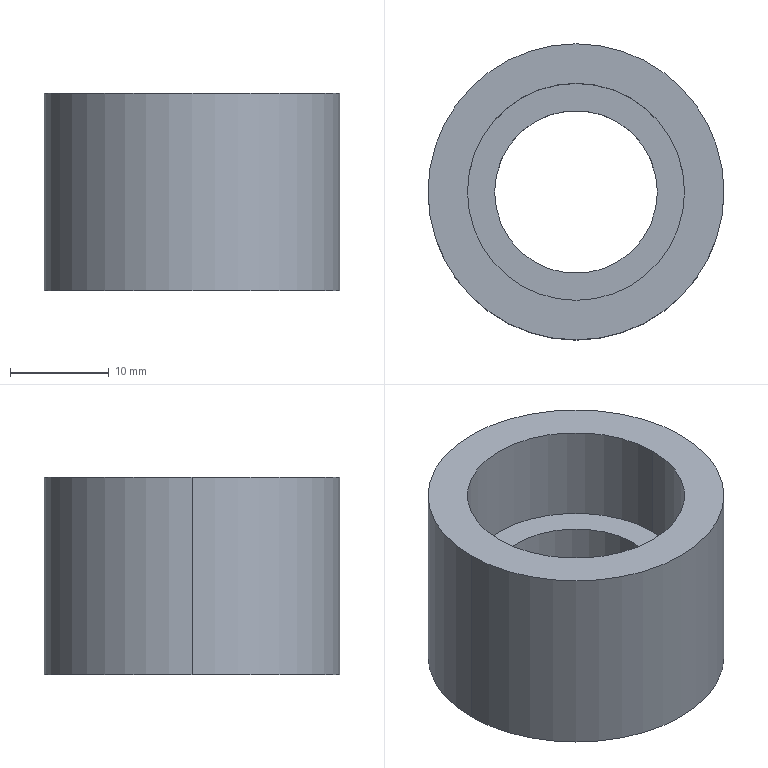Part | SolidWorks | features Extrusion 1, HoleWzd 1, ICE 1 | 1 solid | 9 faces | box 30 x 30 x 20 mm | volume 8198 mm3 | cylinder 6 | plane 3 | commonest cylinder face diameters 16.5 x2 22 x2 30 x2
STEP:
#1=CARTESIAN_POINT('',(-8.25,0.,10.));
#2=VERTEX_POINT('',#1);
#3=CARTESIAN_POINT('',(8.25,0.,10.));
#4=VERTEX_POINT('',#3);
#5=CARTESIAN_POINT('',(0.,0.,10.));
#6=DIRECTION('',(0.,0.,1.));
#7=DIRECTION('',(1.,0.,0.));
#8=AXIS2_PLACEMENT_3D('',#5,#6,#7);
#9=CIRCLE('',#8,8.25);
#10=EDGE_CURVE('',#2,#4,#9,.T.);
#11=ORIENTED_EDGE('',*,*,#10,.T.);
#12=CARTESIAN_POINT('',(8.25,0.,0.));
#13=VERTEX_POINT('',#12);
#14=CARTESIAN_POINT('',(8.25,0.,0.));
#15=DIRECTION('',(0.,0.,-1.));
#16=VECTOR('',#15,1000.);
#17=LINE('',#14,#16);
#18=EDGE_CURVE('',#4,#13,#17,.T.);
#19=ORIENTED_EDGE('',*,*,#18,.T.);
#20=CARTESIAN_POINT('',(-8.25,0.,0.));
#21=VERTEX_POINT('',#20);
#22=CARTESIAN_POINT('',(0.,0.,0.));
#23=DIRECTION('',(0.,0.,-1.));
#24=DIRECTION('',(-1.,0.,0.));
#25=AXIS2_PLACEMENT_3D('',#22,#23,#24);
#26=CIRCLE('',#25,8.25);
#27=EDGE_CURVE('',#13,#21,#26,.T.);
#28=ORIENTED_EDGE('',*,*,#27,.T.);
#29=CARTESIAN_POINT('',(-8.25,0.,0.));
#30=DIRECTION('',(0.,0.,-1.));
#31=VECTOR('',#30,1000.);
#32=LINE('',#29,#31);
#33=EDGE_CURVE('',#2,#21,#32,.T.);
#34=ORIENTED_EDGE('',*,*,#33,.F.);
#35=EDGE_LOOP('',(#11,#19,#28,#34));
#36=FACE_OUTER_BOUND('',#35,.T.);
#37=CARTESIAN_POINT('',(0.,0.,0.));
#38=DIRECTION('',(0.,0.,-1.));
#39=DIRECTION('',(-1.,0.,0.));
#40=AXIS2_PLACEMENT_3D('',#37,#38,#39);
#41=CYLINDRICAL_SURFACE('',#40,8.25);
#42=ADVANCED_FACE('',(#36),#41,.F.);
#43=CARTESIAN_POINT('',(-11.,0.,10.));
#44=VERTEX_POINT('',#43);
#45=CARTESIAN_POINT('',(11.,0.,10.));
#46=VERTEX_POINT('',#45);
#47=CARTESIAN_POINT('',(0.,0.,10.));
#48=DIRECTION('',(0.,0.,1.));
#49=DIRECTION('',(1.,0.,0.));
#50=AXIS2_PLACEMENT_3D('',#47,#48,#49);
#51=CIRCLE('',#50,11.);
#52=EDGE_CURVE('',#44,#46,#51,.T.);
#53=ORIENTED_EDGE('',*,*,#52,.F.);
#54=CARTESIAN_POINT('',(-11.,0.,20.));
#55=VERTEX_POINT('',#54);
#56=CARTESIAN_POINT('',(-11.,0.,10.));
#57=DIRECTION('',(0.,0.,1.));
#58=VECTOR('',#57,1000.);
#59=LINE('',#56,#58);
#60=EDGE_CURVE('',#44,#55,#59,.T.);
#61=ORIENTED_EDGE('',*,*,#60,.T.);
#62=CARTESIAN_POINT('',(11.,0.,20.));
#63=VERTEX_POINT('',#62);
#64=CARTESIAN_POINT('',(0.,0.,20.));
#65=DIRECTION('',(0.,0.,1.));
#66=DIRECTION('',(1.,0.,0.));
#67=AXIS2_PLACEMENT_3D('',#64,#65,#66);
#68=CIRCLE('',#67,11.);
#69=EDGE_CURVE('',#55,#63,#68,.T.);
#70=ORIENTED_EDGE('',*,*,#69,.T.);
#71=CARTESIAN_POINT('',(11.,0.,10.));
#72=DIRECTION('',(0.,0.,1.));
#73=VECTOR('',#72,1000.);
#74=LINE('',#71,#73);
#75=EDGE_CURVE('',#46,#63,#74,.T.);
#76=ORIENTED_EDGE('',*,*,#75,.F.);
#77=EDGE_LOOP('',(#53,#61,#70,#76));
#78=FACE_OUTER_BOUND('',#77,.T.);
#79=CARTESIAN_POINT('',(0.,0.,10.));
#80=DIRECTION('',(0.,0.,1.));
#81=DIRECTION('',(1.,0.,0.));
#82=AXIS2_PLACEMENT_3D('',#79,#80,#81);
#83=CYLINDRICAL_SURFACE('',#82,11.);
#84=ADVANCED_FACE('',(#78),#83,.F.);
#85=CARTESIAN_POINT('',(15.,0.,20.));
#86=VERTEX_POINT('',#85);
#87=CARTESIAN_POINT('',(-15.,0.,20.));
#88=VERTEX_POINT('',#87);
#89=CARTESIAN_POINT('',(0.,0.,20.));
#90=DIRECTION('',(0.,0.,1.));
#91=DIRECTION('',(1.,0.,0.));
#92=AXIS2_PLACEMENT_3D('',#89,#90,#91);
#93=CIRCLE('',#92,15.);
#94=EDGE_CURVE('',#86,#88,#93,.T.);
#95=ORIENTED_EDGE('',*,*,#94,.F.);
#96=CARTESIAN_POINT('',(15.,0.,0.));
#97=VERTEX_POINT('',#96);
#98=CARTESIAN_POINT('',(15.,0.,20.));
#99=DIRECTION('',(0.,0.,-1.));
#100=VECTOR('',#99,1000.);
#101=LINE('',#98,#100);
#102=EDGE_CURVE('',#86,#97,#101,.T.);
#103=ORIENTED_EDGE('',*,*,#102,.T.);
#104=CARTESIAN_POINT('',(-15.,0.,0.));
#105=VERTEX_POINT('',#104);
#106=CARTESIAN_POINT('',(0.,0.,0.));
#107=DIRECTION('',(0.,0.,1.));
#108=DIRECTION('',(1.,0.,0.));
#109=AXIS2_PLACEMENT_3D('',#106,#107,#108);
#110=CIRCLE('',#109,15.);
#111=EDGE_CURVE('',#97,#105,#110,.T.);
#112=ORIENTED_EDGE('',*,*,#111,.T.);
#113=CARTESIAN_POINT('',(-15.,0.,20.));
#114=DIRECTION('',(0.,0.,-1.));
#115=VECTOR('',#114,1000.);
#116=LINE('',#113,#115);
#117=EDGE_CURVE('',#88,#105,#116,.T.);
#118=ORIENTED_EDGE('',*,*,#117,.F.);
#119=EDGE_LOOP('',(#95,#103,#112,#118));
#120=FACE_OUTER_BOUND('',#119,.T.);
#121=CARTESIAN_POINT('',(0.,0.,20.));
#122=DIRECTION('',(0.,0.,-1.));
#123=DIRECTION('',(-1.,0.,0.));
#124=AXIS2_PLACEMENT_3D('',#121,#122,#123);
#125=CYLINDRICAL_SURFACE('',#124,15.);
#126=ADVANCED_FACE('',(#120),#125,.T.);
#127=ORIENTED_EDGE('',*,*,#102,.F.);
#128=CARTESIAN_POINT('',(0.,0.,20.));
#129=DIRECTION('',(0.,0.,1.));
#130=DIRECTION('',(1.,0.,0.));
#131=AXIS2_PLACEMENT_3D('',#128,#129,#130);
#132=CIRCLE('',#131,15.);
#133=EDGE_CURVE('',#88,#86,#132,.T.);
#134=ORIENTED_EDGE('',*,*,#133,.F.);
#135=ORIENTED_EDGE('',*,*,#117,.T.);
#136=CARTESIAN_POINT('',(0.,0.,0.));
#137=DIRECTION('',(0.,0.,1.));
#138=DIRECTION('',(1.,0.,0.));
#139=AXIS2_PLACEMENT_3D('',#136,#137,#138);
#140=CIRCLE('',#139,15.);
#141=EDGE_CURVE('',#105,#97,#140,.T.);
#142=ORIENTED_EDGE('',*,*,#141,.T.);
#143=EDGE_LOOP('',(#127,#134,#135,#142));
#144=FACE_OUTER_BOUND('',#143,.T.);
#145=CARTESIAN_POINT('',(0.,0.,20.));
#146=DIRECTION('',(0.,0.,-1.));
#147=DIRECTION('',(-1.,0.,0.));
#148=AXIS2_PLACEMENT_3D('',#145,#146,#147);
#149=CYLINDRICAL_SURFACE('',#148,15.);
#150=ADVANCED_FACE('',(#144),#149,.T.);
#151=CARTESIAN_POINT('',(0.,0.,20.));
#152=DIRECTION('',(0.,0.,1.));
#153=DIRECTION('',(1.,0.,0.));
#154=AXIS2_PLACEMENT_3D('',#151,#152,#153);
#155=CIRCLE('',#154,11.);
#156=EDGE_CURVE('',#63,#55,#155,.T.);
#157=ORIENTED_EDGE('',*,*,#156,.F.);
#158=ORIENTED_EDGE('',*,*,#69,.F.);
#159=EDGE_LOOP('',(#157,#158));
#160=FACE_BOUND('',#159,.T.);
#161=ORIENTED_EDGE('',*,*,#133,.T.);
#162=ORIENTED_EDGE('',*,*,#94,.T.);
#163=EDGE_LOOP('',(#161,#162));
#164=FACE_OUTER_BOUND('',#163,.T.);
#165=CARTESIAN_POINT('',(0.,0.,20.));
#166=DIRECTION('',(0.,0.,1.));
#167=DIRECTION('',(1.,0.,0.));
#168=AXIS2_PLACEMENT_3D('',#165,#166,#167);
#169=PLANE('',#168);
#170=ADVANCED_FACE('',(#160,#164),#169,.T.);
#171=CARTESIAN_POINT('',(0.,0.,0.));
#172=DIRECTION('',(0.,0.,-1.));
#173=DIRECTION('',(-1.,0.,0.));
#174=AXIS2_PLACEMENT_3D('',#171,#172,#173);
#175=CIRCLE('',#174,8.25);
#176=EDGE_CURVE('',#21,#13,#175,.T.);
#177=ORIENTED_EDGE('',*,*,#176,.F.);
#178=ORIENTED_EDGE('',*,*,#27,.F.);
#179=EDGE_LOOP('',(#177,#178));
#180=FACE_BOUND('',#179,.T.);
#181=ORIENTED_EDGE('',*,*,#141,.F.);
#182=ORIENTED_EDGE('',*,*,#111,.F.);
#183=EDGE_LOOP('',(#181,#182));
#184=FACE_OUTER_BOUND('',#183,.T.);
#185=CARTESIAN_POINT('',(0.,0.,0.));
#186=DIRECTION('',(0.,0.,1.));
#187=DIRECTION('',(1.,0.,0.));
#188=AXIS2_PLACEMENT_3D('',#185,#186,#187);
#189=PLANE('',#188);
#190=ADVANCED_FACE('',(#180,#184),#189,.F.);
#191=ORIENTED_EDGE('',*,*,#60,.F.);
#192=CARTESIAN_POINT('',(0.,0.,10.));
#193=DIRECTION('',(0.,0.,1.));
#194=DIRECTION('',(1.,0.,0.));
#195=AXIS2_PLACEMENT_3D('',#192,#193,#194);
#196=CIRCLE('',#195,11.);
#197=EDGE_CURVE('',#46,#44,#196,.T.);
#198=ORIENTED_EDGE('',*,*,#197,.F.);
#199=ORIENTED_EDGE('',*,*,#75,.T.);
#200=ORIENTED_EDGE('',*,*,#156,.T.);
#201=EDGE_LOOP('',(#191,#198,#199,#200));
#202=FACE_OUTER_BOUND('',#201,.T.);
#203=CARTESIAN_POINT('',(0.,0.,10.));
#204=DIRECTION('',(0.,0.,1.));
#205=DIRECTION('',(1.,0.,0.));
#206=AXIS2_PLACEMENT_3D('',#203,#204,#205);
#207=CYLINDRICAL_SURFACE('',#206,11.);
#208=ADVANCED_FACE('',(#202),#207,.F.);
#209=ORIENTED_EDGE('',*,*,#10,.F.);
#210=CARTESIAN_POINT('',(0.,0.,10.));
#211=DIRECTION('',(0.,0.,1.));
#212=DIRECTION('',(1.,0.,0.));
#213=AXIS2_PLACEMENT_3D('',#210,#211,#212);
#214=CIRCLE('',#213,8.25);
#215=EDGE_CURVE('',#4,#2,#214,.T.);
#216=ORIENTED_EDGE('',*,*,#215,.F.);
#217=EDGE_LOOP('',(#209,#216));
#218=FACE_BOUND('',#217,.T.);
#219=ORIENTED_EDGE('',*,*,#197,.T.);
#220=ORIENTED_EDGE('',*,*,#52,.T.);
#221=EDGE_LOOP('',(#219,#220));
#222=FACE_OUTER_BOUND('',#221,.T.);
#223=CARTESIAN_POINT('',(0.,0.,10.));
#224=DIRECTION('',(0.,0.,1.));
#225=DIRECTION('',(1.,0.,0.));
#226=AXIS2_PLACEMENT_3D('',#223,#224,#225);
#227=PLANE('',#226);
#228=ADVANCED_FACE('',(#218,#222),#227,.T.);
#229=ORIENTED_EDGE('',*,*,#18,.F.);
#230=ORIENTED_EDGE('',*,*,#215,.T.);
#231=ORIENTED_EDGE('',*,*,#33,.T.);
#232=ORIENTED_EDGE('',*,*,#176,.T.);
#233=EDGE_LOOP('',(#229,#230,#231,#232));
#234=FACE_OUTER_BOUND('',#233,.T.);
#235=CARTESIAN_POINT('',(0.,0.,0.));
#236=DIRECTION('',(0.,0.,-1.));
#237=DIRECTION('',(-1.,0.,0.));
#238=AXIS2_PLACEMENT_3D('',#235,#236,#237);
#239=CYLINDRICAL_SURFACE('',#238,8.25);
#240=ADVANCED_FACE('',(#234),#239,.F.);
#241=CLOSED_SHELL('',(#42,#84,#126,#150,#170,#190,#208,#228,#240));
#242=MANIFOLD_SOLID_BREP('',#241);
#243=CARTESIAN_POINT('',(0.,0.,0.));
#244=DIRECTION('',(0.,0.,1.));
#245=DIRECTION('',(1.,0.,0.));
#246=AXIS2_PLACEMENT_3D('',#243,#244,#245);
#247=(LENGTH_UNIT()NAMED_UNIT(*)SI_UNIT(.MILLI.,.METRE.));
#248=UNCERTAINTY_MEASURE_WITH_UNIT(LENGTH_MEASURE(0.00001),#247,'','');
#249=(NAMED_UNIT(*)PLANE_ANGLE_UNIT()SI_UNIT($,.RADIAN.));
#250=(NAMED_UNIT(*)SI_UNIT($,.STERADIAN.)SOLID_ANGLE_UNIT());
#251=(GEOMETRIC_REPRESENTATION_CONTEXT(3)GLOBAL_UNCERTAINTY_ASSIGNED_CONTEXT((#248))GLOBAL_UNIT_ASSIGNED_CONTEXT((#247,#249,#250))REPRESENTATION_CONTEXT('',''));
#252=ADVANCED_BREP_SHAPE_REPRESENTATION('',(#242,#246),#251);